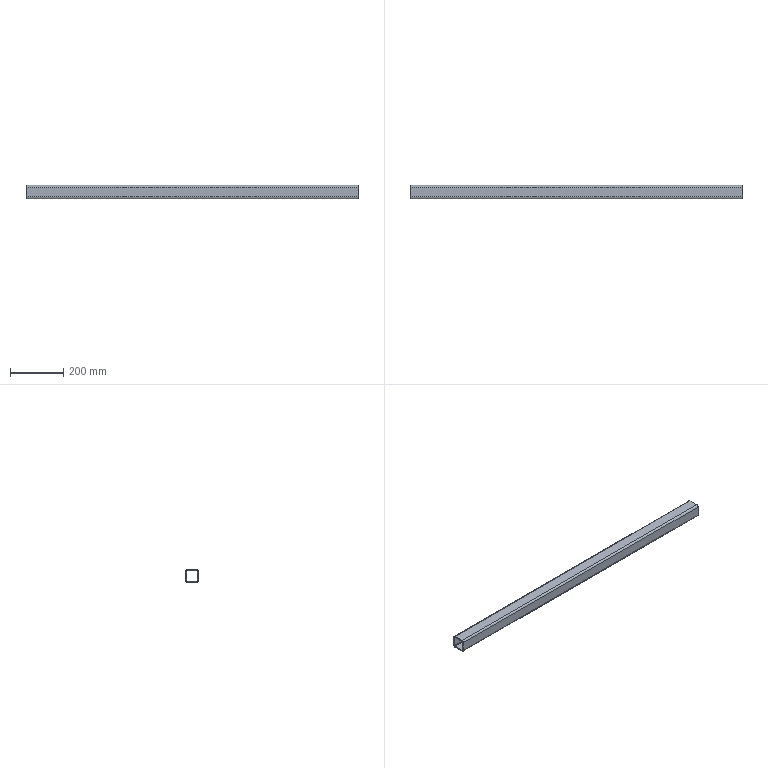Part | NX | 1 solid | 18 faces | box 1250 x 50 x 50 mm | volume 1076715 mm3 | plane 10 | cylinder 8 | commonest cylinder face diameters 4 x4 14 x4
STEP:
#1=CARTESIAN_POINT('',(-950.,874.,-370.));
#2=VERTEX_POINT('',#1);
#3=CARTESIAN_POINT('',(300.,874.,-370.));
#4=VERTEX_POINT('',#3);
#5=CARTESIAN_POINT('',(-975.,874.,-370.));
#6=DIRECTION('',(1.,0.,0.));
#7=VECTOR('',#6,1000.);
#8=LINE('',#5,#7);
#9=EDGE_CURVE('',#2,#4,#8,.T.);
#10=ORIENTED_EDGE('',*,*,#9,.F.);
#11=CARTESIAN_POINT('',(-950.,838.,-370.));
#12=VERTEX_POINT('',#11);
#13=CARTESIAN_POINT('',(-950.,838.,-370.));
#14=DIRECTION('',(0.,-1.,0.));
#15=VECTOR('',#14,1000.);
#16=LINE('',#13,#15);
#17=EDGE_CURVE('',#2,#12,#16,.T.);
#18=ORIENTED_EDGE('',*,*,#17,.T.);
#19=CARTESIAN_POINT('',(300.,838.,-370.));
#20=VERTEX_POINT('',#19);
#21=CARTESIAN_POINT('',(-975.,838.,-370.));
#22=DIRECTION('',(1.,0.,0.));
#23=VECTOR('',#22,1000.);
#24=LINE('',#21,#23);
#25=EDGE_CURVE('',#12,#20,#24,.T.);
#26=ORIENTED_EDGE('',*,*,#25,.T.);
#27=CARTESIAN_POINT('',(300.,838.,-370.));
#28=DIRECTION('',(0.,1.,0.));
#29=VECTOR('',#28,1000.);
#30=LINE('',#27,#29);
#31=EDGE_CURVE('',#20,#4,#30,.T.);
#32=ORIENTED_EDGE('',*,*,#31,.T.);
#33=EDGE_LOOP('',(#10,#18,#26,#32));
#34=FACE_BOUND('',#33,.T.);
#35=CARTESIAN_POINT('',(-975.,838.,-370.));
#36=DIRECTION('',(0.,0.,1.));
#37=DIRECTION('',(0.,-1.,0.));
#38=AXIS2_PLACEMENT_3D('',#35,#36,#37);
#39=PLANE('',#38);
#40=ADVANCED_FACE('',(#34),#39,.T.);
#41=ORIENTED_EDGE('',*,*,#25,.F.);
#42=CARTESIAN_POINT('',(-950.,836.,-368.));
#43=VERTEX_POINT('',#42);
#44=CARTESIAN_POINT('',(-950.,838.,-368.));
#45=DIRECTION('',(-1.,0.,0.));
#46=DIRECTION('',(0.,-1.,0.));
#47=AXIS2_PLACEMENT_3D('',#44,#45,#46);
#48=CIRCLE('',#47,2.);
#49=EDGE_CURVE('',#12,#43,#48,.T.);
#50=ORIENTED_EDGE('',*,*,#49,.T.);
#51=CARTESIAN_POINT('',(300.,836.,-368.));
#52=VERTEX_POINT('',#51);
#53=CARTESIAN_POINT('',(-975.,836.,-368.));
#54=DIRECTION('',(1.,0.,0.));
#55=VECTOR('',#54,1000.);
#56=LINE('',#53,#55);
#57=EDGE_CURVE('',#43,#52,#56,.T.);
#58=ORIENTED_EDGE('',*,*,#57,.T.);
#59=CARTESIAN_POINT('',(300.,838.,-368.));
#60=DIRECTION('',(1.,0.,0.));
#61=DIRECTION('',(0.,1.,0.));
#62=AXIS2_PLACEMENT_3D('',#59,#60,#61);
#63=CIRCLE('',#62,2.);
#64=EDGE_CURVE('',#52,#20,#63,.T.);
#65=ORIENTED_EDGE('',*,*,#64,.T.);
#66=EDGE_LOOP('',(#41,#50,#58,#65));
#67=FACE_BOUND('',#66,.T.);
#68=CARTESIAN_POINT('',(-975.,838.,-368.));
#69=DIRECTION('',(1.,0.,0.));
#70=DIRECTION('',(0.,0.,-1.));
#71=AXIS2_PLACEMENT_3D('',#68,#69,#70);
#72=CYLINDRICAL_SURFACE('',#71,2.);
#73=ADVANCED_FACE('',(#67),#72,.F.);
#74=ORIENTED_EDGE('',*,*,#57,.F.);
#75=CARTESIAN_POINT('',(-950.,836.,-332.));
#76=VERTEX_POINT('',#75);
#77=CARTESIAN_POINT('',(-950.,836.,-368.));
#78=DIRECTION('',(0.,0.,1.));
#79=VECTOR('',#78,1000.);
#80=LINE('',#77,#79);
#81=EDGE_CURVE('',#43,#76,#80,.T.);
#82=ORIENTED_EDGE('',*,*,#81,.T.);
#83=CARTESIAN_POINT('',(300.,836.,-332.));
#84=VERTEX_POINT('',#83);
#85=CARTESIAN_POINT('',(-975.,836.,-332.));
#86=DIRECTION('',(1.,0.,0.));
#87=VECTOR('',#86,1000.);
#88=LINE('',#85,#87);
#89=EDGE_CURVE('',#76,#84,#88,.T.);
#90=ORIENTED_EDGE('',*,*,#89,.T.);
#91=CARTESIAN_POINT('',(300.,836.,-368.));
#92=DIRECTION('',(0.,0.,-1.));
#93=VECTOR('',#92,1000.);
#94=LINE('',#91,#93);
#95=EDGE_CURVE('',#84,#52,#94,.T.);
#96=ORIENTED_EDGE('',*,*,#95,.T.);
#97=EDGE_LOOP('',(#74,#82,#90,#96));
#98=FACE_BOUND('',#97,.T.);
#99=CARTESIAN_POINT('',(-975.,836.,-368.));
#100=DIRECTION('',(0.,1.,0.));
#101=DIRECTION('',(0.,0.,1.));
#102=AXIS2_PLACEMENT_3D('',#99,#100,#101);
#103=PLANE('',#102);
#104=ADVANCED_FACE('',(#98),#103,.T.);
#105=ORIENTED_EDGE('',*,*,#89,.F.);
#106=CARTESIAN_POINT('',(-950.,838.,-330.));
#107=VERTEX_POINT('',#106);
#108=CARTESIAN_POINT('',(-950.,838.,-332.));
#109=DIRECTION('',(-1.,0.,0.));
#110=DIRECTION('',(0.,-1.,0.));
#111=AXIS2_PLACEMENT_3D('',#108,#109,#110);
#112=CIRCLE('',#111,2.);
#113=EDGE_CURVE('',#76,#107,#112,.T.);
#114=ORIENTED_EDGE('',*,*,#113,.T.);
#115=CARTESIAN_POINT('',(300.,838.,-330.));
#116=VERTEX_POINT('',#115);
#117=CARTESIAN_POINT('',(-975.,838.,-330.));
#118=DIRECTION('',(1.,0.,0.));
#119=VECTOR('',#118,1000.);
#120=LINE('',#117,#119);
#121=EDGE_CURVE('',#107,#116,#120,.T.);
#122=ORIENTED_EDGE('',*,*,#121,.T.);
#123=CARTESIAN_POINT('',(300.,838.,-332.));
#124=DIRECTION('',(1.,0.,0.));
#125=DIRECTION('',(0.,1.,0.));
#126=AXIS2_PLACEMENT_3D('',#123,#124,#125);
#127=CIRCLE('',#126,2.);
#128=EDGE_CURVE('',#116,#84,#127,.T.);
#129=ORIENTED_EDGE('',*,*,#128,.T.);
#130=EDGE_LOOP('',(#105,#114,#122,#129));
#131=FACE_BOUND('',#130,.T.);
#132=CARTESIAN_POINT('',(-975.,838.,-332.));
#133=DIRECTION('',(1.,0.,0.));
#134=DIRECTION('',(0.,0.,-1.));
#135=AXIS2_PLACEMENT_3D('',#132,#133,#134);
#136=CYLINDRICAL_SURFACE('',#135,2.);
#137=ADVANCED_FACE('',(#131),#136,.F.);
#138=ORIENTED_EDGE('',*,*,#121,.F.);
#139=CARTESIAN_POINT('',(-950.,874.,-330.));
#140=VERTEX_POINT('',#139);
#141=CARTESIAN_POINT('',(-950.,874.,-330.));
#142=DIRECTION('',(0.,1.,0.));
#143=VECTOR('',#142,1000.);
#144=LINE('',#141,#143);
#145=EDGE_CURVE('',#107,#140,#144,.T.);
#146=ORIENTED_EDGE('',*,*,#145,.T.);
#147=CARTESIAN_POINT('',(300.,874.,-330.));
#148=VERTEX_POINT('',#147);
#149=CARTESIAN_POINT('',(-975.,874.,-330.));
#150=DIRECTION('',(1.,0.,0.));
#151=VECTOR('',#150,1000.);
#152=LINE('',#149,#151);
#153=EDGE_CURVE('',#140,#148,#152,.T.);
#154=ORIENTED_EDGE('',*,*,#153,.T.);
#155=CARTESIAN_POINT('',(300.,874.,-330.));
#156=DIRECTION('',(0.,-1.,0.));
#157=VECTOR('',#156,1000.);
#158=LINE('',#155,#157);
#159=EDGE_CURVE('',#148,#116,#158,.T.);
#160=ORIENTED_EDGE('',*,*,#159,.T.);
#161=EDGE_LOOP('',(#138,#146,#154,#160));
#162=FACE_BOUND('',#161,.T.);
#163=CARTESIAN_POINT('',(-975.,874.,-330.));
#164=DIRECTION('',(0.,0.,-1.));
#165=DIRECTION('',(0.,1.,0.));
#166=AXIS2_PLACEMENT_3D('',#163,#164,#165);
#167=PLANE('',#166);
#168=ADVANCED_FACE('',(#162),#167,.T.);
#169=ORIENTED_EDGE('',*,*,#153,.F.);
#170=CARTESIAN_POINT('',(-950.,876.,-332.));
#171=VERTEX_POINT('',#170);
#172=CARTESIAN_POINT('',(-950.,874.,-332.));
#173=DIRECTION('',(-1.,0.,0.));
#174=DIRECTION('',(0.,-1.,0.));
#175=AXIS2_PLACEMENT_3D('',#172,#173,#174);
#176=CIRCLE('',#175,2.);
#177=EDGE_CURVE('',#140,#171,#176,.T.);
#178=ORIENTED_EDGE('',*,*,#177,.T.);
#179=CARTESIAN_POINT('',(300.,876.,-332.));
#180=VERTEX_POINT('',#179);
#181=CARTESIAN_POINT('',(-975.,876.,-332.));
#182=DIRECTION('',(1.,0.,0.));
#183=VECTOR('',#182,1000.);
#184=LINE('',#181,#183);
#185=EDGE_CURVE('',#171,#180,#184,.T.);
#186=ORIENTED_EDGE('',*,*,#185,.T.);
#187=CARTESIAN_POINT('',(300.,874.,-332.));
#188=DIRECTION('',(1.,0.,0.));
#189=DIRECTION('',(0.,1.,0.));
#190=AXIS2_PLACEMENT_3D('',#187,#188,#189);
#191=CIRCLE('',#190,2.);
#192=EDGE_CURVE('',#180,#148,#191,.T.);
#193=ORIENTED_EDGE('',*,*,#192,.T.);
#194=EDGE_LOOP('',(#169,#178,#186,#193));
#195=FACE_BOUND('',#194,.T.);
#196=CARTESIAN_POINT('',(-975.,874.,-332.));
#197=DIRECTION('',(1.,0.,0.));
#198=DIRECTION('',(0.,0.,-1.));
#199=AXIS2_PLACEMENT_3D('',#196,#197,#198);
#200=CYLINDRICAL_SURFACE('',#199,2.);
#201=ADVANCED_FACE('',(#195),#200,.F.);
#202=ORIENTED_EDGE('',*,*,#185,.F.);
#203=CARTESIAN_POINT('',(-950.,876.,-368.));
#204=VERTEX_POINT('',#203);
#205=CARTESIAN_POINT('',(-950.,876.,-332.));
#206=DIRECTION('',(0.,0.,-1.));
#207=VECTOR('',#206,1000.);
#208=LINE('',#205,#207);
#209=EDGE_CURVE('',#171,#204,#208,.T.);
#210=ORIENTED_EDGE('',*,*,#209,.T.);
#211=CARTESIAN_POINT('',(300.,876.,-368.));
#212=VERTEX_POINT('',#211);
#213=CARTESIAN_POINT('',(-975.,876.,-368.));
#214=DIRECTION('',(1.,0.,0.));
#215=VECTOR('',#214,1000.);
#216=LINE('',#213,#215);
#217=EDGE_CURVE('',#204,#212,#216,.T.);
#218=ORIENTED_EDGE('',*,*,#217,.T.);
#219=CARTESIAN_POINT('',(300.,876.,-332.));
#220=DIRECTION('',(0.,0.,1.));
#221=VECTOR('',#220,1000.);
#222=LINE('',#219,#221);
#223=EDGE_CURVE('',#212,#180,#222,.T.);
#224=ORIENTED_EDGE('',*,*,#223,.T.);
#225=EDGE_LOOP('',(#202,#210,#218,#224));
#226=FACE_BOUND('',#225,.T.);
#227=CARTESIAN_POINT('',(-975.,876.,-332.));
#228=DIRECTION('',(0.,-1.,0.));
#229=DIRECTION('',(0.,0.,-1.));
#230=AXIS2_PLACEMENT_3D('',#227,#228,#229);
#231=PLANE('',#230);
#232=ADVANCED_FACE('',(#226),#231,.T.);
#233=ORIENTED_EDGE('',*,*,#217,.F.);
#234=CARTESIAN_POINT('',(-950.,874.,-368.));
#235=DIRECTION('',(-1.,0.,0.));
#236=DIRECTION('',(0.,-1.,0.));
#237=AXIS2_PLACEMENT_3D('',#234,#235,#236);
#238=CIRCLE('',#237,2.);
#239=EDGE_CURVE('',#204,#2,#238,.T.);
#240=ORIENTED_EDGE('',*,*,#239,.T.);
#241=ORIENTED_EDGE('',*,*,#9,.T.);
#242=CARTESIAN_POINT('',(300.,874.,-368.));
#243=DIRECTION('',(1.,0.,0.));
#244=DIRECTION('',(0.,1.,0.));
#245=AXIS2_PLACEMENT_3D('',#242,#243,#244);
#246=CIRCLE('',#245,2.);
#247=EDGE_CURVE('',#4,#212,#246,.T.);
#248=ORIENTED_EDGE('',*,*,#247,.T.);
#249=EDGE_LOOP('',(#233,#240,#241,#248));
#250=FACE_BOUND('',#249,.T.);
#251=CARTESIAN_POINT('',(-975.,874.,-368.));
#252=DIRECTION('',(1.,0.,0.));
#253=DIRECTION('',(0.,0.,-1.));
#254=AXIS2_PLACEMENT_3D('',#251,#252,#253);
#255=CYLINDRICAL_SURFACE('',#254,2.);
#256=ADVANCED_FACE('',(#250),#255,.F.);
#257=CARTESIAN_POINT('',(-950.,838.,-325.));
#258=VERTEX_POINT('',#257);
#259=CARTESIAN_POINT('',(-950.,874.,-325.));
#260=VERTEX_POINT('',#259);
#261=CARTESIAN_POINT('',(-950.,874.,-325.));
#262=DIRECTION('',(0.,1.,0.));
#263=VECTOR('',#262,1000.);
#264=LINE('',#261,#263);
#265=EDGE_CURVE('',#258,#260,#264,.T.);
#266=ORIENTED_EDGE('',*,*,#265,.F.);
#267=CARTESIAN_POINT('',(300.,838.,-325.));
#268=VERTEX_POINT('',#267);
#269=CARTESIAN_POINT('',(-975.,838.,-325.));
#270=DIRECTION('',(1.,0.,0.));
#271=VECTOR('',#270,1000.);
#272=LINE('',#269,#271);
#273=EDGE_CURVE('',#258,#268,#272,.T.);
#274=ORIENTED_EDGE('',*,*,#273,.T.);
#275=CARTESIAN_POINT('',(300.,874.,-325.));
#276=VERTEX_POINT('',#275);
#277=CARTESIAN_POINT('',(300.,874.,-325.));
#278=DIRECTION('',(0.,-1.,0.));
#279=VECTOR('',#278,1000.);
#280=LINE('',#277,#279);
#281=EDGE_CURVE('',#276,#268,#280,.T.);
#282=ORIENTED_EDGE('',*,*,#281,.F.);
#283=CARTESIAN_POINT('',(-975.,874.,-325.));
#284=DIRECTION('',(1.,0.,0.));
#285=VECTOR('',#284,1000.);
#286=LINE('',#283,#285);
#287=EDGE_CURVE('',#260,#276,#286,.T.);
#288=ORIENTED_EDGE('',*,*,#287,.F.);
#289=EDGE_LOOP('',(#266,#274,#282,#288));
#290=FACE_BOUND('',#289,.T.);
#291=CARTESIAN_POINT('',(-975.,874.,-325.));
#292=DIRECTION('',(0.,0.,-1.));
#293=DIRECTION('',(0.,1.,0.));
#294=AXIS2_PLACEMENT_3D('',#291,#292,#293);
#295=PLANE('',#294);
#296=ADVANCED_FACE('',(#290),#295,.F.);
#297=CARTESIAN_POINT('',(-950.,831.,-332.));
#298=VERTEX_POINT('',#297);
#299=CARTESIAN_POINT('',(-950.,838.,-332.));
#300=DIRECTION('',(-1.,0.,0.));
#301=DIRECTION('',(0.,-1.,0.));
#302=AXIS2_PLACEMENT_3D('',#299,#300,#301);
#303=CIRCLE('',#302,7.);
#304=EDGE_CURVE('',#298,#258,#303,.T.);
#305=ORIENTED_EDGE('',*,*,#304,.F.);
#306=CARTESIAN_POINT('',(300.,831.,-332.));
#307=VERTEX_POINT('',#306);
#308=CARTESIAN_POINT('',(-975.,831.,-332.));
#309=DIRECTION('',(1.,0.,0.));
#310=VECTOR('',#309,1000.);
#311=LINE('',#308,#310);
#312=EDGE_CURVE('',#298,#307,#311,.T.);
#313=ORIENTED_EDGE('',*,*,#312,.T.);
#314=CARTESIAN_POINT('',(300.,838.,-332.));
#315=DIRECTION('',(1.,0.,0.));
#316=DIRECTION('',(0.,1.,0.));
#317=AXIS2_PLACEMENT_3D('',#314,#315,#316);
#318=CIRCLE('',#317,7.);
#319=EDGE_CURVE('',#268,#307,#318,.T.);
#320=ORIENTED_EDGE('',*,*,#319,.F.);
#321=ORIENTED_EDGE('',*,*,#273,.F.);
#322=EDGE_LOOP('',(#305,#313,#320,#321));
#323=FACE_BOUND('',#322,.T.);
#324=CARTESIAN_POINT('',(-975.,838.,-332.));
#325=DIRECTION('',(1.,0.,0.));
#326=DIRECTION('',(0.,0.,-1.));
#327=AXIS2_PLACEMENT_3D('',#324,#325,#326);
#328=CYLINDRICAL_SURFACE('',#327,7.);
#329=ADVANCED_FACE('',(#323),#328,.T.);
#330=CARTESIAN_POINT('',(-950.,831.,-368.));
#331=VERTEX_POINT('',#330);
#332=CARTESIAN_POINT('',(-950.,831.,575.));
#333=DIRECTION('',(0.,0.,-1.));
#334=VECTOR('',#333,1000.);
#335=LINE('',#332,#334);
#336=EDGE_CURVE('',#298,#331,#335,.T.);
#337=ORIENTED_EDGE('',*,*,#336,.T.);
#338=CARTESIAN_POINT('',(300.,831.,-368.));
#339=VERTEX_POINT('',#338);
#340=CARTESIAN_POINT('',(-975.,831.,-368.));
#341=DIRECTION('',(1.,0.,0.));
#342=VECTOR('',#341,1000.);
#343=LINE('',#340,#342);
#344=EDGE_CURVE('',#331,#339,#343,.T.);
#345=ORIENTED_EDGE('',*,*,#344,.T.);
#346=CARTESIAN_POINT('',(300.,831.,575.));
#347=DIRECTION('',(0.,0.,-1.));
#348=VECTOR('',#347,1000.);
#349=LINE('',#346,#348);
#350=EDGE_CURVE('',#307,#339,#349,.T.);
#351=ORIENTED_EDGE('',*,*,#350,.F.);
#352=ORIENTED_EDGE('',*,*,#312,.F.);
#353=EDGE_LOOP('',(#337,#345,#351,#352));
#354=FACE_BOUND('',#353,.T.);
#355=CARTESIAN_POINT('',(-975.,831.,-368.));
#356=DIRECTION('',(0.,1.,0.));
#357=DIRECTION('',(0.,0.,1.));
#358=AXIS2_PLACEMENT_3D('',#355,#356,#357);
#359=PLANE('',#358);
#360=ADVANCED_FACE('',(#354),#359,.F.);
#361=CARTESIAN_POINT('',(-950.,838.,-375.));
#362=VERTEX_POINT('',#361);
#363=CARTESIAN_POINT('',(-950.,838.,-368.));
#364=DIRECTION('',(-1.,0.,0.));
#365=DIRECTION('',(0.,-1.,0.));
#366=AXIS2_PLACEMENT_3D('',#363,#364,#365);
#367=CIRCLE('',#366,7.);
#368=EDGE_CURVE('',#362,#331,#367,.T.);
#369=ORIENTED_EDGE('',*,*,#368,.F.);
#370=CARTESIAN_POINT('',(300.,838.,-375.));
#371=VERTEX_POINT('',#370);
#372=CARTESIAN_POINT('',(-975.,838.,-375.));
#373=DIRECTION('',(1.,0.,0.));
#374=VECTOR('',#373,1000.);
#375=LINE('',#372,#374);
#376=EDGE_CURVE('',#362,#371,#375,.T.);
#377=ORIENTED_EDGE('',*,*,#376,.T.);
#378=CARTESIAN_POINT('',(300.,838.,-368.));
#379=DIRECTION('',(1.,0.,0.));
#380=DIRECTION('',(0.,1.,0.));
#381=AXIS2_PLACEMENT_3D('',#378,#379,#380);
#382=CIRCLE('',#381,7.);
#383=EDGE_CURVE('',#339,#371,#382,.T.);
#384=ORIENTED_EDGE('',*,*,#383,.F.);
#385=ORIENTED_EDGE('',*,*,#344,.F.);
#386=EDGE_LOOP('',(#369,#377,#384,#385));
#387=FACE_BOUND('',#386,.T.);
#388=CARTESIAN_POINT('',(-975.,838.,-368.));
#389=DIRECTION('',(1.,0.,0.));
#390=DIRECTION('',(0.,0.,-1.));
#391=AXIS2_PLACEMENT_3D('',#388,#389,#390);
#392=CYLINDRICAL_SURFACE('',#391,7.);
#393=ADVANCED_FACE('',(#387),#392,.T.);
#394=CARTESIAN_POINT('',(-950.,874.,-375.));
#395=VERTEX_POINT('',#394);
#396=CARTESIAN_POINT('',(-950.,838.,-375.));
#397=DIRECTION('',(0.,-1.,0.));
#398=VECTOR('',#397,1000.);
#399=LINE('',#396,#398);
#400=EDGE_CURVE('',#395,#362,#399,.T.);
#401=ORIENTED_EDGE('',*,*,#400,.F.);
#402=CARTESIAN_POINT('',(300.,874.,-375.));
#403=VERTEX_POINT('',#402);
#404=CARTESIAN_POINT('',(-975.,874.,-375.));
#405=DIRECTION('',(1.,0.,0.));
#406=VECTOR('',#405,1000.);
#407=LINE('',#404,#406);
#408=EDGE_CURVE('',#395,#403,#407,.T.);
#409=ORIENTED_EDGE('',*,*,#408,.T.);
#410=CARTESIAN_POINT('',(300.,838.,-375.));
#411=DIRECTION('',(0.,1.,0.));
#412=VECTOR('',#411,1000.);
#413=LINE('',#410,#412);
#414=EDGE_CURVE('',#371,#403,#413,.T.);
#415=ORIENTED_EDGE('',*,*,#414,.F.);
#416=ORIENTED_EDGE('',*,*,#376,.F.);
#417=EDGE_LOOP('',(#401,#409,#415,#416));
#418=FACE_BOUND('',#417,.T.);
#419=CARTESIAN_POINT('',(-975.,838.,-375.));
#420=DIRECTION('',(0.,0.,1.));
#421=DIRECTION('',(0.,-1.,0.));
#422=AXIS2_PLACEMENT_3D('',#419,#420,#421);
#423=PLANE('',#422);
#424=ADVANCED_FACE('',(#418),#423,.F.);
#425=CARTESIAN_POINT('',(-950.,881.,-368.));
#426=VERTEX_POINT('',#425);
#427=CARTESIAN_POINT('',(-950.,874.,-368.));
#428=DIRECTION('',(-1.,0.,0.));
#429=DIRECTION('',(0.,-1.,0.));
#430=AXIS2_PLACEMENT_3D('',#427,#428,#429);
#431=CIRCLE('',#430,7.);
#432=EDGE_CURVE('',#426,#395,#431,.T.);
#433=ORIENTED_EDGE('',*,*,#432,.F.);
#434=CARTESIAN_POINT('',(300.,881.,-368.));
#435=VERTEX_POINT('',#434);
#436=CARTESIAN_POINT('',(-975.,881.,-368.));
#437=DIRECTION('',(1.,0.,0.));
#438=VECTOR('',#437,1000.);
#439=LINE('',#436,#438);
#440=EDGE_CURVE('',#426,#435,#439,.T.);
#441=ORIENTED_EDGE('',*,*,#440,.T.);
#442=CARTESIAN_POINT('',(300.,874.,-368.));
#443=DIRECTION('',(1.,0.,0.));
#444=DIRECTION('',(0.,1.,0.));
#445=AXIS2_PLACEMENT_3D('',#442,#443,#444);
#446=CIRCLE('',#445,7.);
#447=EDGE_CURVE('',#403,#435,#446,.T.);
#448=ORIENTED_EDGE('',*,*,#447,.F.);
#449=ORIENTED_EDGE('',*,*,#408,.F.);
#450=EDGE_LOOP('',(#433,#441,#448,#449));
#451=FACE_BOUND('',#450,.T.);
#452=CARTESIAN_POINT('',(-975.,874.,-368.));
#453=DIRECTION('',(1.,0.,0.));
#454=DIRECTION('',(0.,0.,-1.));
#455=AXIS2_PLACEMENT_3D('',#452,#453,#454);
#456=CYLINDRICAL_SURFACE('',#455,7.);
#457=ADVANCED_FACE('',(#451),#456,.T.);
#458=CARTESIAN_POINT('',(-950.,881.,-332.));
#459=VERTEX_POINT('',#458);
#460=CARTESIAN_POINT('',(-950.,881.,575.));
#461=DIRECTION('',(0.,0.,-1.));
#462=VECTOR('',#461,1000.);
#463=LINE('',#460,#462);
#464=EDGE_CURVE('',#459,#426,#463,.T.);
#465=ORIENTED_EDGE('',*,*,#464,.F.);
#466=CARTESIAN_POINT('',(300.,881.,-332.));
#467=VERTEX_POINT('',#466);
#468=CARTESIAN_POINT('',(-975.,881.,-332.));
#469=DIRECTION('',(1.,0.,0.));
#470=VECTOR('',#469,1000.);
#471=LINE('',#468,#470);
#472=EDGE_CURVE('',#459,#467,#471,.T.);
#473=ORIENTED_EDGE('',*,*,#472,.T.);
#474=CARTESIAN_POINT('',(300.,881.,575.));
#475=DIRECTION('',(0.,0.,-1.));
#476=VECTOR('',#475,1000.);
#477=LINE('',#474,#476);
#478=EDGE_CURVE('',#467,#435,#477,.T.);
#479=ORIENTED_EDGE('',*,*,#478,.T.);
#480=ORIENTED_EDGE('',*,*,#440,.F.);
#481=EDGE_LOOP('',(#465,#473,#479,#480));
#482=FACE_BOUND('',#481,.T.);
#483=CARTESIAN_POINT('',(-975.,881.,-332.));
#484=DIRECTION('',(0.,-1.,0.));
#485=DIRECTION('',(0.,0.,-1.));
#486=AXIS2_PLACEMENT_3D('',#483,#484,#485);
#487=PLANE('',#486);
#488=ADVANCED_FACE('',(#482),#487,.F.);
#489=CARTESIAN_POINT('',(-950.,874.,-332.));
#490=DIRECTION('',(-1.,0.,0.));
#491=DIRECTION('',(0.,-1.,0.));
#492=AXIS2_PLACEMENT_3D('',#489,#490,#491);
#493=CIRCLE('',#492,7.);
#494=EDGE_CURVE('',#260,#459,#493,.T.);
#495=ORIENTED_EDGE('',*,*,#494,.F.);
#496=ORIENTED_EDGE('',*,*,#287,.T.);
#497=CARTESIAN_POINT('',(300.,874.,-332.));
#498=DIRECTION('',(1.,0.,0.));
#499=DIRECTION('',(0.,1.,0.));
#500=AXIS2_PLACEMENT_3D('',#497,#498,#499);
#501=CIRCLE('',#500,7.);
#502=EDGE_CURVE('',#467,#276,#501,.T.);
#503=ORIENTED_EDGE('',*,*,#502,.F.);
#504=ORIENTED_EDGE('',*,*,#472,.F.);
#505=EDGE_LOOP('',(#495,#496,#503,#504));
#506=FACE_BOUND('',#505,.T.);
#507=CARTESIAN_POINT('',(-975.,874.,-332.));
#508=DIRECTION('',(1.,0.,0.));
#509=DIRECTION('',(0.,0.,-1.));
#510=AXIS2_PLACEMENT_3D('',#507,#508,#509);
#511=CYLINDRICAL_SURFACE('',#510,7.);
#512=ADVANCED_FACE('',(#506),#511,.T.);
#513=ORIENTED_EDGE('',*,*,#31,.F.);
#514=ORIENTED_EDGE('',*,*,#64,.F.);
#515=ORIENTED_EDGE('',*,*,#95,.F.);
#516=ORIENTED_EDGE('',*,*,#128,.F.);
#517=ORIENTED_EDGE('',*,*,#159,.F.);
#518=ORIENTED_EDGE('',*,*,#192,.F.);
#519=ORIENTED_EDGE('',*,*,#223,.F.);
#520=ORIENTED_EDGE('',*,*,#247,.F.);
#521=EDGE_LOOP('',(#513,#514,#515,#516,#517,#518,#519,#520));
#522=FACE_BOUND('',#521,.T.);
#523=ORIENTED_EDGE('',*,*,#447,.T.);
#524=ORIENTED_EDGE('',*,*,#478,.F.);
#525=ORIENTED_EDGE('',*,*,#502,.T.);
#526=ORIENTED_EDGE('',*,*,#281,.T.);
#527=ORIENTED_EDGE('',*,*,#319,.T.);
#528=ORIENTED_EDGE('',*,*,#350,.T.);
#529=ORIENTED_EDGE('',*,*,#383,.T.);
#530=ORIENTED_EDGE('',*,*,#414,.T.);
#531=EDGE_LOOP('',(#523,#524,#525,#526,#527,#528,#529,#530));
#532=FACE_BOUND('',#531,.T.);
#533=CARTESIAN_POINT('',(300.,838.,575.));
#534=DIRECTION('',(1.,0.,0.));
#535=DIRECTION('',(0.,1.,0.));
#536=AXIS2_PLACEMENT_3D('',#533,#534,#535);
#537=PLANE('',#536);
#538=ADVANCED_FACE('',(#522,#532),#537,.T.);
#539=ORIENTED_EDGE('',*,*,#239,.F.);
#540=ORIENTED_EDGE('',*,*,#209,.F.);
#541=ORIENTED_EDGE('',*,*,#177,.F.);
#542=ORIENTED_EDGE('',*,*,#145,.F.);
#543=ORIENTED_EDGE('',*,*,#113,.F.);
#544=ORIENTED_EDGE('',*,*,#81,.F.);
#545=ORIENTED_EDGE('',*,*,#49,.F.);
#546=ORIENTED_EDGE('',*,*,#17,.F.);
#547=EDGE_LOOP('',(#539,#540,#541,#542,#543,#544,#545,#546));
#548=FACE_BOUND('',#547,.T.);
#549=ORIENTED_EDGE('',*,*,#368,.T.);
#550=ORIENTED_EDGE('',*,*,#336,.F.);
#551=ORIENTED_EDGE('',*,*,#304,.T.);
#552=ORIENTED_EDGE('',*,*,#265,.T.);
#553=ORIENTED_EDGE('',*,*,#494,.T.);
#554=ORIENTED_EDGE('',*,*,#464,.T.);
#555=ORIENTED_EDGE('',*,*,#432,.T.);
#556=ORIENTED_EDGE('',*,*,#400,.T.);
#557=EDGE_LOOP('',(#549,#550,#551,#552,#553,#554,#555,#556));
#558=FACE_BOUND('',#557,.T.);
#559=CARTESIAN_POINT('',(-950.,874.,575.));
#560=DIRECTION('',(-1.,0.,0.));
#561=DIRECTION('',(0.,-1.,0.));
#562=AXIS2_PLACEMENT_3D('',#559,#560,#561);
#563=PLANE('',#562);
#564=ADVANCED_FACE('',(#548,#558),#563,.T.);
#565=CLOSED_SHELL('',(#40,#73,#104,#137,#168,#201,#232,#256,#296,#329,#360,#393,#424,#457,#488,#512,#538,#564));
#566=MANIFOLD_SOLID_BREP('',#565);
#567=(LENGTH_UNIT()NAMED_UNIT(*)SI_UNIT(.MILLI.,.METRE.));
#568=UNCERTAINTY_MEASURE_WITH_UNIT(LENGTH_MEASURE(0.00001),#567,'','');
#569=(NAMED_UNIT(*)PLANE_ANGLE_UNIT()SI_UNIT($,.RADIAN.));
#570=(NAMED_UNIT(*)SI_UNIT($,.STERADIAN.)SOLID_ANGLE_UNIT());
#571=(GEOMETRIC_REPRESENTATION_CONTEXT(3)GLOBAL_UNCERTAINTY_ASSIGNED_CONTEXT((#568))GLOBAL_UNIT_ASSIGNED_CONTEXT((#567,#569,#570))REPRESENTATION_CONTEXT('',''));
#572=ADVANCED_BREP_SHAPE_REPRESENTATION('',(#566),#571);